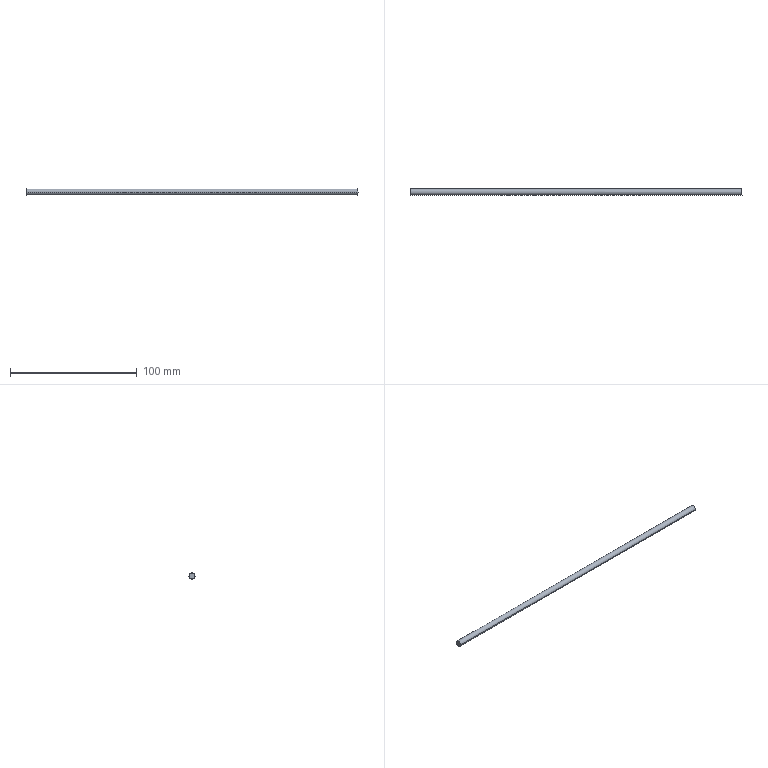Part | Creo | 1 solid | 4 faces | box 262 x 4.8 x 4.8 mm | volume 4741 mm3 | plane 2 | cylinder 2 | commonest cylinder face diameters 4.8 x2
STEP:
#1=CARTESIAN_POINT('',(-332.,-180.08,92.4));
#2=VERTEX_POINT('',#1);
#3=CARTESIAN_POINT('',(-332.,-177.68,90.));
#4=VERTEX_POINT('',#3);
#5=CARTESIAN_POINT('',(-332.,-180.08,90.));
#6=DIRECTION('',(-1.,0.,0.));
#7=DIRECTION('',(0.,0.,1.));
#8=AXIS2_PLACEMENT_3D('',#5,#6,#7);
#9=CIRCLE('',#8,2.4);
#10=EDGE_CURVE('',#2,#4,#9,.T.);
#11=ORIENTED_EDGE('',*,*,#10,.F.);
#12=CARTESIAN_POINT('',(-332.,-182.48,90.));
#13=VERTEX_POINT('',#12);
#14=CARTESIAN_POINT('',(-332.,-180.08,90.));
#15=DIRECTION('',(-1.,0.,0.));
#16=DIRECTION('',(0.,-1.,0.));
#17=AXIS2_PLACEMENT_3D('',#14,#15,#16);
#18=CIRCLE('',#17,2.4);
#19=EDGE_CURVE('',#13,#2,#18,.T.);
#20=ORIENTED_EDGE('',*,*,#19,.F.);
#21=CARTESIAN_POINT('',(-332.,-180.08,87.6));
#22=VERTEX_POINT('',#21);
#23=CARTESIAN_POINT('',(-332.,-180.08,90.));
#24=DIRECTION('',(-1.,0.,0.));
#25=DIRECTION('',(0.,0.,-1.));
#26=AXIS2_PLACEMENT_3D('',#23,#24,#25);
#27=CIRCLE('',#26,2.4);
#28=EDGE_CURVE('',#22,#13,#27,.T.);
#29=ORIENTED_EDGE('',*,*,#28,.F.);
#30=CARTESIAN_POINT('',(-332.,-180.08,90.));
#31=DIRECTION('',(-1.,0.,0.));
#32=DIRECTION('',(0.,1.,0.));
#33=AXIS2_PLACEMENT_3D('',#30,#31,#32);
#34=CIRCLE('',#33,2.4);
#35=EDGE_CURVE('',#4,#22,#34,.T.);
#36=ORIENTED_EDGE('',*,*,#35,.F.);
#37=EDGE_LOOP('',(#11,#20,#29,#36));
#38=FACE_OUTER_BOUND('',#37,.F.);
#39=CARTESIAN_POINT('',(-332.,-180.08,90.));
#40=DIRECTION('',(-1.,0.,0.));
#41=DIRECTION('',(0.,0.,1.));
#42=AXIS2_PLACEMENT_3D('',#39,#40,#41);
#43=PLANE('',#42);
#44=ADVANCED_FACE('',(#38),#43,.T.);
#45=CARTESIAN_POINT('',(-70.,-177.68,90.));
#46=VERTEX_POINT('',#45);
#47=CARTESIAN_POINT('',(-70.,-182.48,90.));
#48=VERTEX_POINT('',#47);
#49=CARTESIAN_POINT('',(-70.,-180.08,90.));
#50=DIRECTION('',(1.,0.,0.));
#51=DIRECTION('',(0.,1.,0.));
#52=AXIS2_PLACEMENT_3D('',#49,#50,#51);
#53=CIRCLE('',#52,2.4);
#54=EDGE_CURVE('',#46,#48,#53,.T.);
#55=ORIENTED_EDGE('',*,*,#54,.T.);
#56=CARTESIAN_POINT('',(-332.,-182.48,90.));
#57=DIRECTION('',(1.,0.,0.));
#58=VECTOR('',#57,262.);
#59=LINE('',#56,#58);
#60=EDGE_CURVE('',#13,#48,#59,.T.);
#61=ORIENTED_EDGE('',*,*,#60,.F.);
#62=ORIENTED_EDGE('',*,*,#19,.T.);
#63=ORIENTED_EDGE('',*,*,#10,.T.);
#64=CARTESIAN_POINT('',(-332.,-177.68,90.));
#65=DIRECTION('',(1.,0.,0.));
#66=VECTOR('',#65,262.);
#67=LINE('',#64,#66);
#68=EDGE_CURVE('',#4,#46,#67,.T.);
#69=ORIENTED_EDGE('',*,*,#68,.T.);
#70=EDGE_LOOP('',(#55,#61,#62,#63,#69));
#71=FACE_OUTER_BOUND('',#70,.F.);
#72=CARTESIAN_POINT('',(-99.,-180.08,90.));
#73=DIRECTION('',(1.,0.,0.));
#74=DIRECTION('',(0.,1.,0.));
#75=AXIS2_PLACEMENT_3D('',#72,#73,#74);
#76=CYLINDRICAL_SURFACE('',#75,2.4);
#77=ADVANCED_FACE('',(#71),#76,.T.);
#78=CARTESIAN_POINT('',(-70.,-180.08,90.));
#79=DIRECTION('',(1.,0.,0.));
#80=DIRECTION('',(0.,-1.,0.));
#81=AXIS2_PLACEMENT_3D('',#78,#79,#80);
#82=CIRCLE('',#81,2.4);
#83=EDGE_CURVE('',#48,#46,#82,.T.);
#84=ORIENTED_EDGE('',*,*,#83,.F.);
#85=ORIENTED_EDGE('',*,*,#54,.F.);
#86=EDGE_LOOP('',(#84,#85));
#87=FACE_OUTER_BOUND('',#86,.F.);
#88=CARTESIAN_POINT('',(-70.,-2.967,45.5));
#89=DIRECTION('',(-1.,-0.000000059,0.));
#90=DIRECTION('',(0.000000059,-1.,0.));
#91=AXIS2_PLACEMENT_3D('',#88,#89,#90);
#92=PLANE('',#91);
#93=ADVANCED_FACE('',(#87),#92,.F.);
#94=ORIENTED_EDGE('',*,*,#83,.T.);
#95=ORIENTED_EDGE('',*,*,#68,.F.);
#96=ORIENTED_EDGE('',*,*,#35,.T.);
#97=ORIENTED_EDGE('',*,*,#28,.T.);
#98=ORIENTED_EDGE('',*,*,#60,.T.);
#99=EDGE_LOOP('',(#94,#95,#96,#97,#98));
#100=FACE_OUTER_BOUND('',#99,.F.);
#101=CARTESIAN_POINT('',(-99.,-180.08,90.));
#102=DIRECTION('',(1.,0.,0.));
#103=DIRECTION('',(0.,1.,0.));
#104=AXIS2_PLACEMENT_3D('',#101,#102,#103);
#105=CYLINDRICAL_SURFACE('',#104,2.4);
#106=ADVANCED_FACE('',(#100),#105,.T.);
#107=CLOSED_SHELL('',(#44,#77,#93,#106));
#108=MANIFOLD_SOLID_BREP('',#107);
#109=(LENGTH_UNIT()NAMED_UNIT(*)SI_UNIT(.MILLI.,.METRE.));
#110=UNCERTAINTY_MEASURE_WITH_UNIT(LENGTH_MEASURE(0.02621),#109,'','');
#111=(NAMED_UNIT(*)PLANE_ANGLE_UNIT()SI_UNIT($,.RADIAN.));
#112=PLANE_ANGLE_MEASURE_WITH_UNIT(PLANE_ANGLE_MEASURE(0.01745),#111);
#113=(CONVERSION_BASED_UNIT('DEGREE',#112)NAMED_UNIT(*)PLANE_ANGLE_UNIT());
#114=(NAMED_UNIT(*)SI_UNIT($,.STERADIAN.)SOLID_ANGLE_UNIT());
#115=(GEOMETRIC_REPRESENTATION_CONTEXT(3)GLOBAL_UNCERTAINTY_ASSIGNED_CONTEXT((#110))GLOBAL_UNIT_ASSIGNED_CONTEXT((#109,#113,#114))REPRESENTATION_CONTEXT('',''));
#116=ADVANCED_BREP_SHAPE_REPRESENTATION('',(#108),#115);